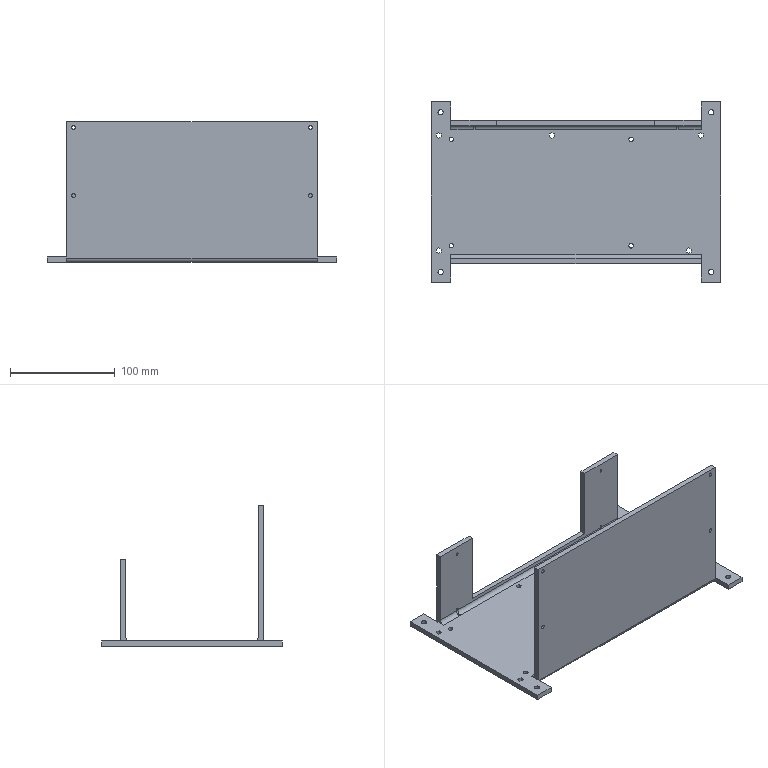Part | NX | features BREP 1 | 1 solid | 80 faces | box 276 x 172 x 134 mm | volume 387826 mm3 | plane 56 | cylinder 22 | spline 2 | commonest cylinder face diameters 8 x6 2.5 x4 3.6 x4 4.3 x4 5 x4